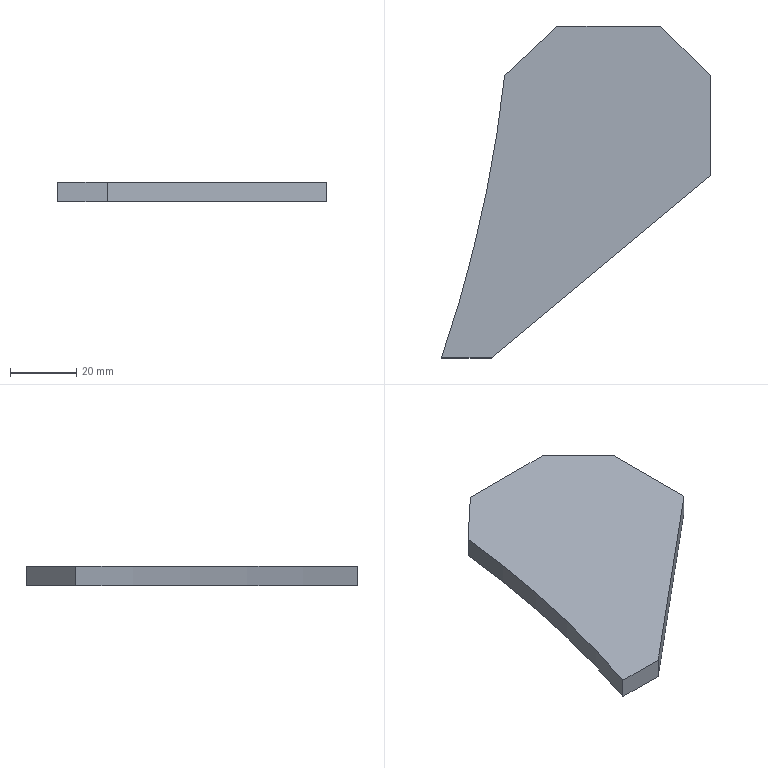Part | SolidWorks | features Extrusion 1 | 1 solid | 9 faces | box 81 x 100 x 6 mm | volume 28941 mm3 | plane 8 | cylinder 1 | commonest cylinder face diameters 810 x1
STEP:
#1=CARTESIAN_POINT('',(19.,85.,0.));
#2=VERTEX_POINT('',#1);
#3=CARTESIAN_POINT('',(0.,0.,0.));
#4=VERTEX_POINT('',#3);
#5=CARTESIAN_POINT('',(-383.454,130.337,0.));
#6=DIRECTION('',(0.,0.,-1.));
#7=DIRECTION('',(-1.,0.,0.));
#8=AXIS2_PLACEMENT_3D('',#5,#6,#7);
#9=CIRCLE('',#8,405.);
#10=EDGE_CURVE('',#2,#4,#9,.T.);
#11=ORIENTED_EDGE('',*,*,#10,.T.);
#12=CARTESIAN_POINT('',(0.,0.,6.));
#13=VERTEX_POINT('',#12);
#14=CARTESIAN_POINT('',(0.,0.,6.));
#15=DIRECTION('',(0.,0.,-1.));
#16=VECTOR('',#15,1000.);
#17=LINE('',#14,#16);
#18=EDGE_CURVE('',#13,#4,#17,.T.);
#19=ORIENTED_EDGE('',*,*,#18,.F.);
#20=CARTESIAN_POINT('',(19.,85.,6.));
#21=VERTEX_POINT('',#20);
#22=CARTESIAN_POINT('',(-383.454,130.337,6.));
#23=DIRECTION('',(0.,0.,-1.));
#24=DIRECTION('',(-1.,0.,0.));
#25=AXIS2_PLACEMENT_3D('',#22,#23,#24);
#26=CIRCLE('',#25,405.);
#27=EDGE_CURVE('',#21,#13,#26,.T.);
#28=ORIENTED_EDGE('',*,*,#27,.F.);
#29=CARTESIAN_POINT('',(19.,85.,6.));
#30=DIRECTION('',(0.,0.,-1.));
#31=VECTOR('',#30,1000.);
#32=LINE('',#29,#31);
#33=EDGE_CURVE('',#21,#2,#32,.T.);
#34=ORIENTED_EDGE('',*,*,#33,.T.);
#35=EDGE_LOOP('',(#11,#19,#28,#34));
#36=FACE_OUTER_BOUND('',#35,.T.);
#37=CARTESIAN_POINT('',(-383.454,130.337,6.));
#38=DIRECTION('',(0.,0.,-1.));
#39=DIRECTION('',(-1.,0.,0.));
#40=AXIS2_PLACEMENT_3D('',#37,#38,#39);
#41=CYLINDRICAL_SURFACE('',#40,405.);
#42=ADVANCED_FACE('',(#36),#41,.F.);
#43=CARTESIAN_POINT('',(15.,0.,0.));
#44=VERTEX_POINT('',#43);
#45=CARTESIAN_POINT('',(0.,0.,0.));
#46=DIRECTION('',(1.,0.,0.));
#47=VECTOR('',#46,1000.);
#48=LINE('',#45,#47);
#49=EDGE_CURVE('',#4,#44,#48,.T.);
#50=ORIENTED_EDGE('',*,*,#49,.T.);
#51=CARTESIAN_POINT('',(15.,0.,6.));
#52=VERTEX_POINT('',#51);
#53=CARTESIAN_POINT('',(15.,0.,6.));
#54=DIRECTION('',(0.,0.,-1.));
#55=VECTOR('',#54,1000.);
#56=LINE('',#53,#55);
#57=EDGE_CURVE('',#52,#44,#56,.T.);
#58=ORIENTED_EDGE('',*,*,#57,.F.);
#59=CARTESIAN_POINT('',(0.,0.,6.));
#60=DIRECTION('',(1.,0.,0.));
#61=VECTOR('',#60,1000.);
#62=LINE('',#59,#61);
#63=EDGE_CURVE('',#13,#52,#62,.T.);
#64=ORIENTED_EDGE('',*,*,#63,.F.);
#65=ORIENTED_EDGE('',*,*,#18,.T.);
#66=EDGE_LOOP('',(#50,#58,#64,#65));
#67=FACE_OUTER_BOUND('',#66,.T.);
#68=CARTESIAN_POINT('',(0.,0.,6.));
#69=DIRECTION('',(0.,1.,0.));
#70=DIRECTION('',(0.,0.,1.));
#71=AXIS2_PLACEMENT_3D('',#68,#69,#70);
#72=PLANE('',#71);
#73=ADVANCED_FACE('',(#67),#72,.F.);
#74=CARTESIAN_POINT('',(81.,55.,0.));
#75=VERTEX_POINT('',#74);
#76=CARTESIAN_POINT('',(15.,0.,0.));
#77=DIRECTION('',(0.7682,0.6402,0.));
#78=VECTOR('',#77,1000.);
#79=LINE('',#76,#78);
#80=EDGE_CURVE('',#44,#75,#79,.T.);
#81=ORIENTED_EDGE('',*,*,#80,.T.);
#82=CARTESIAN_POINT('',(81.,55.,6.));
#83=VERTEX_POINT('',#82);
#84=CARTESIAN_POINT('',(81.,55.,6.));
#85=DIRECTION('',(0.,0.,-1.));
#86=VECTOR('',#85,1000.);
#87=LINE('',#84,#86);
#88=EDGE_CURVE('',#83,#75,#87,.T.);
#89=ORIENTED_EDGE('',*,*,#88,.F.);
#90=CARTESIAN_POINT('',(15.,0.,6.));
#91=DIRECTION('',(0.7682,0.6402,0.));
#92=VECTOR('',#91,1000.);
#93=LINE('',#90,#92);
#94=EDGE_CURVE('',#52,#83,#93,.T.);
#95=ORIENTED_EDGE('',*,*,#94,.F.);
#96=ORIENTED_EDGE('',*,*,#57,.T.);
#97=EDGE_LOOP('',(#81,#89,#95,#96));
#98=FACE_OUTER_BOUND('',#97,.T.);
#99=CARTESIAN_POINT('',(15.,0.,6.));
#100=DIRECTION('',(-0.6402,0.7682,0.));
#101=DIRECTION('',(-0.7682,-0.6402,0.));
#102=AXIS2_PLACEMENT_3D('',#99,#100,#101);
#103=PLANE('',#102);
#104=ADVANCED_FACE('',(#98),#103,.F.);
#105=CARTESIAN_POINT('',(81.,85.,0.));
#106=VERTEX_POINT('',#105);
#107=CARTESIAN_POINT('',(81.,55.,0.));
#108=DIRECTION('',(0.,1.,0.));
#109=VECTOR('',#108,1000.);
#110=LINE('',#107,#109);
#111=EDGE_CURVE('',#75,#106,#110,.T.);
#112=ORIENTED_EDGE('',*,*,#111,.T.);
#113=CARTESIAN_POINT('',(81.,85.,6.));
#114=VERTEX_POINT('',#113);
#115=CARTESIAN_POINT('',(81.,85.,6.));
#116=DIRECTION('',(0.,0.,-1.));
#117=VECTOR('',#116,1000.);
#118=LINE('',#115,#117);
#119=EDGE_CURVE('',#114,#106,#118,.T.);
#120=ORIENTED_EDGE('',*,*,#119,.F.);
#121=CARTESIAN_POINT('',(81.,55.,6.));
#122=DIRECTION('',(0.,1.,0.));
#123=VECTOR('',#122,1000.);
#124=LINE('',#121,#123);
#125=EDGE_CURVE('',#83,#114,#124,.T.);
#126=ORIENTED_EDGE('',*,*,#125,.F.);
#127=ORIENTED_EDGE('',*,*,#88,.T.);
#128=EDGE_LOOP('',(#112,#120,#126,#127));
#129=FACE_OUTER_BOUND('',#128,.T.);
#130=CARTESIAN_POINT('',(81.,55.,6.));
#131=DIRECTION('',(-1.,0.,0.));
#132=DIRECTION('',(0.,-1.,0.));
#133=AXIS2_PLACEMENT_3D('',#130,#131,#132);
#134=PLANE('',#133);
#135=ADVANCED_FACE('',(#129),#134,.F.);
#136=CARTESIAN_POINT('',(66.,100.,0.));
#137=VERTEX_POINT('',#136);
#138=CARTESIAN_POINT('',(81.,85.,0.));
#139=DIRECTION('',(-0.7071,0.7071,0.));
#140=VECTOR('',#139,1000.);
#141=LINE('',#138,#140);
#142=EDGE_CURVE('',#106,#137,#141,.T.);
#143=ORIENTED_EDGE('',*,*,#142,.T.);
#144=CARTESIAN_POINT('',(66.,100.,6.));
#145=VERTEX_POINT('',#144);
#146=CARTESIAN_POINT('',(66.,100.,6.));
#147=DIRECTION('',(0.,0.,-1.));
#148=VECTOR('',#147,1000.);
#149=LINE('',#146,#148);
#150=EDGE_CURVE('',#145,#137,#149,.T.);
#151=ORIENTED_EDGE('',*,*,#150,.F.);
#152=CARTESIAN_POINT('',(81.,85.,6.));
#153=DIRECTION('',(-0.7071,0.7071,0.));
#154=VECTOR('',#153,1000.);
#155=LINE('',#152,#154);
#156=EDGE_CURVE('',#114,#145,#155,.T.);
#157=ORIENTED_EDGE('',*,*,#156,.F.);
#158=ORIENTED_EDGE('',*,*,#119,.T.);
#159=EDGE_LOOP('',(#143,#151,#157,#158));
#160=FACE_OUTER_BOUND('',#159,.T.);
#161=CARTESIAN_POINT('',(81.,85.,6.));
#162=DIRECTION('',(-0.7071,-0.7071,0.));
#163=DIRECTION('',(0.7071,-0.7071,0.));
#164=AXIS2_PLACEMENT_3D('',#161,#162,#163);
#165=PLANE('',#164);
#166=ADVANCED_FACE('',(#160),#165,.F.);
#167=CARTESIAN_POINT('',(35.,100.,0.));
#168=VERTEX_POINT('',#167);
#169=CARTESIAN_POINT('',(66.,100.,0.));
#170=DIRECTION('',(-1.,0.,0.));
#171=VECTOR('',#170,1000.);
#172=LINE('',#169,#171);
#173=EDGE_CURVE('',#137,#168,#172,.T.);
#174=ORIENTED_EDGE('',*,*,#173,.T.);
#175=CARTESIAN_POINT('',(35.,100.,6.));
#176=VERTEX_POINT('',#175);
#177=CARTESIAN_POINT('',(35.,100.,6.));
#178=DIRECTION('',(0.,0.,-1.));
#179=VECTOR('',#178,1000.);
#180=LINE('',#177,#179);
#181=EDGE_CURVE('',#176,#168,#180,.T.);
#182=ORIENTED_EDGE('',*,*,#181,.F.);
#183=CARTESIAN_POINT('',(66.,100.,6.));
#184=DIRECTION('',(-1.,0.,0.));
#185=VECTOR('',#184,1000.);
#186=LINE('',#183,#185);
#187=EDGE_CURVE('',#145,#176,#186,.T.);
#188=ORIENTED_EDGE('',*,*,#187,.F.);
#189=ORIENTED_EDGE('',*,*,#150,.T.);
#190=EDGE_LOOP('',(#174,#182,#188,#189));
#191=FACE_OUTER_BOUND('',#190,.T.);
#192=CARTESIAN_POINT('',(66.,100.,6.));
#193=DIRECTION('',(0.,-1.,0.));
#194=DIRECTION('',(0.,0.,-1.));
#195=AXIS2_PLACEMENT_3D('',#192,#193,#194);
#196=PLANE('',#195);
#197=ADVANCED_FACE('',(#191),#196,.F.);
#198=CARTESIAN_POINT('',(35.,100.,0.));
#199=DIRECTION('',(-0.7295,-0.6839,0.));
#200=VECTOR('',#199,1000.);
#201=LINE('',#198,#200);
#202=EDGE_CURVE('',#168,#2,#201,.T.);
#203=ORIENTED_EDGE('',*,*,#202,.T.);
#204=ORIENTED_EDGE('',*,*,#33,.F.);
#205=CARTESIAN_POINT('',(35.,100.,6.));
#206=DIRECTION('',(-0.7295,-0.6839,0.));
#207=VECTOR('',#206,1000.);
#208=LINE('',#205,#207);
#209=EDGE_CURVE('',#176,#21,#208,.T.);
#210=ORIENTED_EDGE('',*,*,#209,.F.);
#211=ORIENTED_EDGE('',*,*,#181,.T.);
#212=EDGE_LOOP('',(#203,#204,#210,#211));
#213=FACE_OUTER_BOUND('',#212,.T.);
#214=CARTESIAN_POINT('',(35.,100.,6.));
#215=DIRECTION('',(0.6839,-0.7295,0.));
#216=DIRECTION('',(0.7295,0.6839,0.));
#217=AXIS2_PLACEMENT_3D('',#214,#215,#216);
#218=PLANE('',#217);
#219=ADVANCED_FACE('',(#213),#218,.F.);
#220=ORIENTED_EDGE('',*,*,#27,.T.);
#221=ORIENTED_EDGE('',*,*,#63,.T.);
#222=ORIENTED_EDGE('',*,*,#94,.T.);
#223=ORIENTED_EDGE('',*,*,#125,.T.);
#224=ORIENTED_EDGE('',*,*,#156,.T.);
#225=ORIENTED_EDGE('',*,*,#187,.T.);
#226=ORIENTED_EDGE('',*,*,#209,.T.);
#227=EDGE_LOOP('',(#220,#221,#222,#223,#224,#225,#226));
#228=FACE_OUTER_BOUND('',#227,.T.);
#229=CARTESIAN_POINT('',(-383.454,130.337,6.));
#230=DIRECTION('',(0.,0.,-1.));
#231=DIRECTION('',(-1.,0.,0.));
#232=AXIS2_PLACEMENT_3D('',#229,#230,#231);
#233=PLANE('',#232);
#234=ADVANCED_FACE('',(#228),#233,.F.);
#235=ORIENTED_EDGE('',*,*,#10,.F.);
#236=ORIENTED_EDGE('',*,*,#202,.F.);
#237=ORIENTED_EDGE('',*,*,#173,.F.);
#238=ORIENTED_EDGE('',*,*,#142,.F.);
#239=ORIENTED_EDGE('',*,*,#111,.F.);
#240=ORIENTED_EDGE('',*,*,#80,.F.);
#241=ORIENTED_EDGE('',*,*,#49,.F.);
#242=EDGE_LOOP('',(#235,#236,#237,#238,#239,#240,#241));
#243=FACE_OUTER_BOUND('',#242,.T.);
#244=CARTESIAN_POINT('',(-383.454,130.337,0.));
#245=DIRECTION('',(0.,0.,-1.));
#246=DIRECTION('',(-1.,0.,0.));
#247=AXIS2_PLACEMENT_3D('',#244,#245,#246);
#248=PLANE('',#247);
#249=ADVANCED_FACE('',(#243),#248,.T.);
#250=CLOSED_SHELL('',(#42,#73,#104,#135,#166,#197,#219,#234,#249));
#251=MANIFOLD_SOLID_BREP('',#250);
#252=CARTESIAN_POINT('',(0.,0.,0.));
#253=DIRECTION('',(0.,0.,1.));
#254=DIRECTION('',(1.,0.,0.));
#255=AXIS2_PLACEMENT_3D('',#252,#253,#254);
#256=(LENGTH_UNIT()NAMED_UNIT(*)SI_UNIT(.MILLI.,.METRE.));
#257=UNCERTAINTY_MEASURE_WITH_UNIT(LENGTH_MEASURE(0.00001),#256,'','');
#258=(NAMED_UNIT(*)PLANE_ANGLE_UNIT()SI_UNIT($,.RADIAN.));
#259=(NAMED_UNIT(*)SI_UNIT($,.STERADIAN.)SOLID_ANGLE_UNIT());
#260=(GEOMETRIC_REPRESENTATION_CONTEXT(3)GLOBAL_UNCERTAINTY_ASSIGNED_CONTEXT((#257))GLOBAL_UNIT_ASSIGNED_CONTEXT((#256,#258,#259))REPRESENTATION_CONTEXT('',''));
#261=ADVANCED_BREP_SHAPE_REPRESENTATION('',(#251,#255),#260);